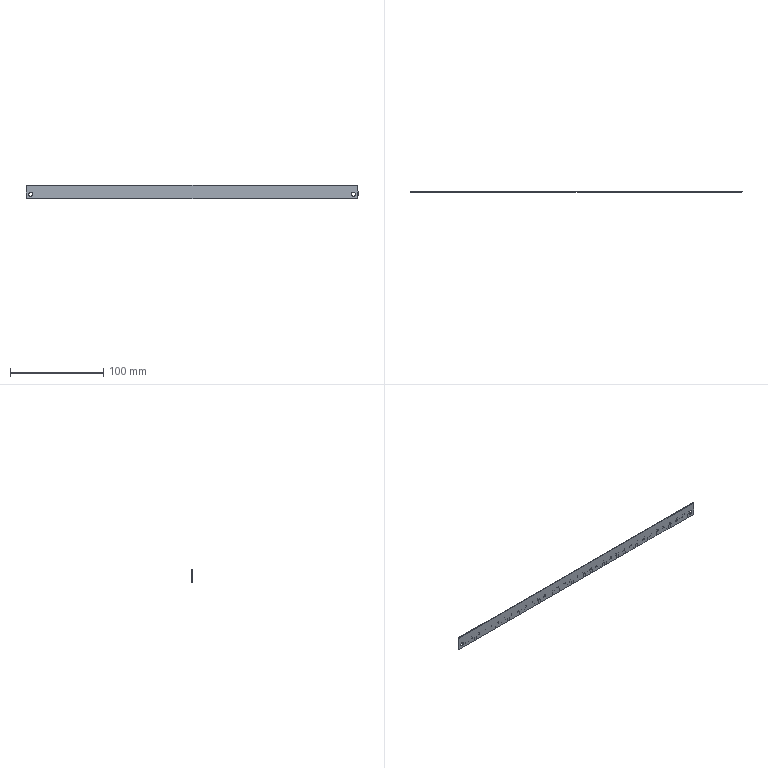Part | SolidWorks | features ICE 5, LPattern 3, Extrusion 1, Fillet 1 | 1 solid | 2306 faces | box 356 x 1 x 15 mm | volume 5253 mm3 | plane 1920 | spline 378 | cylinder 8 | commonest cylinder face diameters 2 x4 4.5 x4